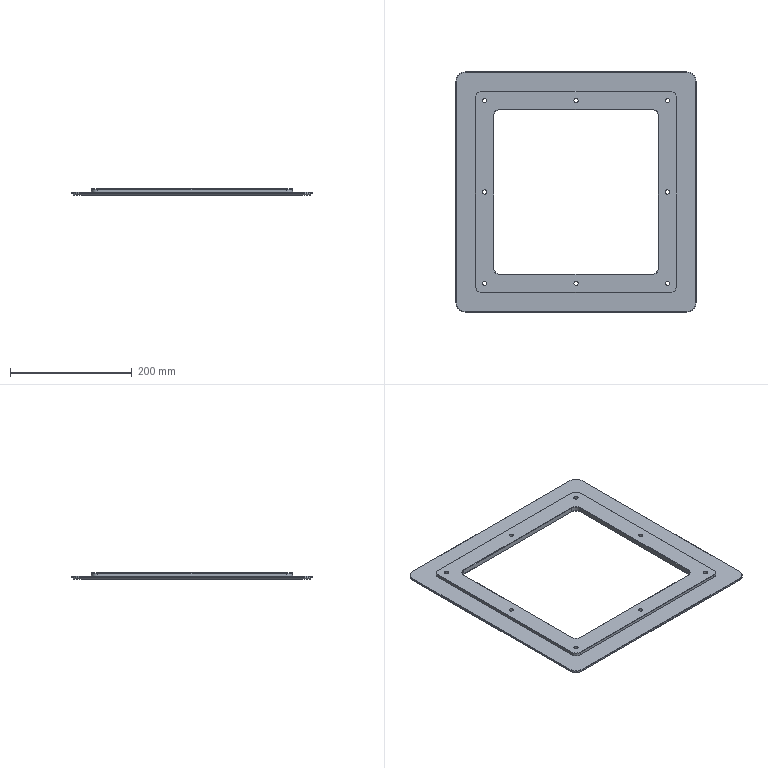NC program | Mastercam | posted with a generic post
Lines 951 to 2441 of 5147:
N9520 T14 M6
N9530 G0 G90 G17 G54 X-266.551 Y206.801 A0. S1600 M3
N9540 G43 H14 Z26.2 M8
N9550 Z11.2
N9560 G1 Z1.017 F1000.
N9570 X-208.008 Y207.805 F3200.
N9580 X208.008
N9590 Y194.817
N9600 X-208.008
N9610 Y181.829
N9620 X208.008
N9630 Y168.841
N9640 X-208.008
N9650 Y155.854
N9660 X208.008
N9670 Y142.866
N9680 X-208.008
N9690 Y129.878
N9700 X208.008
N9710 Y116.89
N9720 X-208.008
N9730 Y103.902
N9740 X-114.974
N9750 G3 X-121.856 Y90.915 I19.974 J-18.902
N9760 G1 X-208.008
N9770 Y77.927
N9780 X-121.575
N9790 G3 X-113.81 Y64.939 I26.575 J7.073
N9800 G1 X-208.008
N9810 Y51.951
N9820 X208.008
N9830 Y38.963
N9840 X-208.008
N9850 Y25.976
N9860 X208.008
N9870 Y12.988
N9880 X-208.008
N9890 Y0.
N9900 X208.008
N9910 Y-12.988
N9920 X-208.008
N9930 Y-25.976
N9940 X208.008
N9950 Y-38.963
N9960 X-208.008
N9970 Y-51.951
N9980 X208.008
N9990 Y-64.939
N100 X113.81
N110 G2 X121.575 Y-77.927 I-18.81 J-20.061
N120 G1 X208.008
N130 Y-90.915
N140 X121.856
N150 G2 X114.974 Y-103.902 I-26.856 J5.915
N160 G1 X208.008
N170 Y-116.89
N180 X-208.008
N190 Y-129.878
N200 X208.008
N210 Y-142.866
N220 X-208.008
N230 Y-155.854
N240 X208.008
N250 Y-168.841
N260 X-208.008
N270 Y-181.829
N280 X208.008
N290 Y-194.817
N300 X-208.008
N310 Y-207.805
N320 X208.008
N330 X81.49 Y-108.953
N340 G2 X75.026 Y-103.902 I13.51 J23.953
N350 G1 X-75.026
N360 G3 X-68.144 Y-90.915 I-19.974 J18.902
N370 G1 X68.144
N380 G2 X67.5 Y-85. I26.856 J5.915
N390 X68.425 Y-77.927 I27.5 J0.
N400 G1 X-68.425
N410 G3 X-76.19 Y-64.939 I-26.575 J-7.073
N420 G1 X76.19
N430 Y64.939
N440 X-76.19
N450 G3 X-68.425 Y77.927 I-18.81 J20.061
N460 G1 X68.425
N470 G2 X67.5 Y85. I26.575 J7.073
N480 X68.144 Y90.915 I27.5 J0.
N490 G1 X-68.144
N500 G3 X-75.026 Y103.902 I-26.856 J-5.915
N510 G1 X75.026
N520 G2 X95. Y112.5 I19.974 J-18.902
N530 X114.974 Y103.902 I0. J-27.5
N540 G1 X208.008
N550 Y90.915
N560 X121.856
N570 G2 X122.5 Y85. I-26.856 J-5.915
N580 X121.575 Y77.927 I-27.5 J0.
N590 G1 X208.008
N600 Y64.939
N610 X113.81
N620 G2 X108.624 Y61.112 I-18.81 J20.061
N630 G1 X-71.049 Y-71.486
N640 G3 X-95. Y-57.499 I-23.951 J-13.514
N650 X-122.501 Y-85. I0. J-27.501
N660 X-114.974 Y-103.902 I27.501 J0.
N670 G1 X-208.008
N680 Y-90.915
N690 X-121.856
N700 G2 X-122.5 Y-85. I26.856 J5.915
N710 X-121.575 Y-77.927 I27.5 J0.
N720 G1 X-208.008
N730 Y-64.939
N740 X-113.81
N750 G0 Z26.017
N760 X-266.551 Y206.801
N770 Z11.017
N780 G1 Z.833 F1000.
N790 X-208.008 Y207.805 F3200.
N800 X208.008
N810 Y194.817
N820 X-208.008
N830 Y181.829
N840 X208.008
N850 Y168.841
N860 X-208.008
N870 Y155.854
N880 X208.008
N890 Y142.866
N900 X-208.008
N910 Y129.878
N920 X208.008
N930 Y116.89
N940 X-208.008
N950 Y103.902
N960 X-114.974
N970 G3 X-121.856 Y90.915 I19.974 J-18.902
N980 G1 X-208.008
N990 Y77.927
N1000 X-121.575
N1010 G3 X-113.81 Y64.939 I26.575 J7.073
N1020 G1 X-208.008
N1030 Y51.951
N1040 X208.008
N1050 Y38.963
N1060 X-208.008
N1070 Y25.976
N1080 X208.008
N1090 Y12.988
N1100 X-208.008
N1110 Y0.
N1120 X208.008
N1130 Y-12.988
N1140 X-208.008
N1150 Y-25.976
N1160 X208.008
N1170 Y-38.963
N1180 X-208.008
N1190 Y-51.951
N1200 X208.008
N1210 Y-64.939
N1220 X113.81
N1230 G2 X121.575 Y-77.927 I-18.81 J-20.061
N1240 G1 X208.008
N1250 Y-90.915
N1260 X121.856
N1270 G2 X114.974 Y-103.902 I-26.856 J5.915
N1280 G1 X208.008
N1290 Y-116.89
N1300 X-208.008
N1310 Y-129.878
N1320 X208.008
N1330 Y-142.866
N1340 X-208.008
N1350 Y-155.854
N1360 X208.008
N1370 Y-168.841
N1380 X-208.008
N1390 Y-181.829
N1400 X208.008
N1410 Y-194.817
N1420 X-208.008
N1430 Y-207.805
N1440 X208.008
N1450 X81.49 Y-108.953
N1460 G2 X75.026 Y-103.902 I13.51 J23.953
N1470 G1 X-75.026
N1480 G3 X-68.144 Y-90.915 I-19.974 J18.902
N1490 G1 X68.144
N1500 G2 X67.5 Y-85. I26.856 J5.915
N1510 X68.425 Y-77.927 I27.5 J0.
N1520 G1 X-68.425
N1530 G3 X-76.19 Y-64.939 I-26.575 J-7.073
N1540 G1 X76.19
N1550 Y64.939
N1560 X-76.19
N1570 G3 X-68.425 Y77.927 I-18.81 J20.061
N1580 G1 X68.425
N1590 G2 X67.5 Y85. I26.575 J7.073
N1600 X68.144 Y90.915 I27.5 J0.
N1610 G1 X-68.144
N1620 G3 X-75.026 Y103.902 I-26.856 J-5.915
N1630 G1 X75.026
N1640 G2 X95. Y112.5 I19.974 J-18.902
N1650 X114.974 Y103.902 I0. J-27.5
N1660 G1 X208.008
N1670 Y90.915
N1680 X121.856
N1690 G2 X122.5 Y85. I-26.856 J-5.915
N1700 X121.575 Y77.927 I-27.5 J0.
N1710 G1 X208.008
N1720 Y64.939
N1730 X113.81
N1740 G2 X108.624 Y61.112 I-18.81 J20.061
N1750 G1 X-71.049 Y-71.486
N1760 G3 X-95. Y-57.499 I-23.951 J-13.514
N1770 X-122.501 Y-85. I0. J-27.501
N1780 X-114.974 Y-103.902 I27.501 J0.
N1790 G1 X-208.008
N1800 Y-90.915
N1810 X-121.856
N1820 G2 X-122.5 Y-85. I26.856 J5.915
N1830 X-121.575 Y-77.927 I27.5 J0.
N1840 G1 X-208.008
N1850 Y-64.939
N1860 X-113.81
N1870 G0 Z25.833
N1880 X-266.551 Y206.801
N1890 Z10.833
N1900 G1 Z.65 F1000.
N1910 X-208.008 Y207.805 F3200.
N1920 X208.008
N1930 Y194.817
N1940 X-208.008
N1950 Y181.829
N1960 X208.008
N1970 Y168.841
N1980 X-208.008
N1990 Y155.854
N2000 X208.008
N2010 Y142.866
N2020 X-208.008
N2030 Y129.878
N2040 X208.008
N2050 Y116.89
N2060 X-208.008
N2070 Y103.902
N2080 X-114.974
N2090 G3 X-121.856 Y90.915 I19.974 J-18.902
N2100 G1 X-208.008
N2110 Y77.927
N2120 X-121.575
N2130 G3 X-113.81 Y64.939 I26.575 J7.073
N2140 G1 X-208.008
N2150 Y51.951
N2160 X208.008
N2170 Y38.963
N2180 X-208.008
N2190 Y25.976
N2200 X208.008
N2210 Y12.988
N2220 X-208.008
N2230 Y0.
N2240 X208.008
N2250 Y-12.988
N2260 X-208.008
N2270 Y-25.976
N2280 X208.008
N2290 Y-38.963
N2300 X-208.008
N2310 Y-51.951
N2320 X208.008
N2330 Y-64.939
N2340 X113.81
N2350 G2 X121.575 Y-77.927 I-18.81 J-20.061
N2360 G1 X208.008
N2370 Y-90.915
N2380 X121.856
N2390 G2 X114.974 Y-103.902 I-26.856 J5.915
N2400 G1 X208.008
N2410 Y-116.89
N2420 X-208.008
N2430 Y-129.878
N2440 X208.008
N2450 Y-142.866
N2460 X-208.008
N2470 Y-155.854
N2480 X208.008
N2490 Y-168.841
N2500 X-208.008
N2510 Y-181.829
N2520 X208.008
N2530 Y-194.817
N2540 X-208.008
N2550 Y-207.805
N2560 X208.008
N2570 X81.49 Y-108.953
N2580 G2 X75.026 Y-103.902 I13.51 J23.953
N2590 G1 X-75.026
N2600 G3 X-68.144 Y-90.915 I-19.974 J18.902
N2610 G1 X68.144
N2620 G2 X67.5 Y-85. I26.856 J5.915
N2630 X68.425 Y-77.927 I27.5 J0.
N2640 G1 X-68.425
N2650 G3 X-76.19 Y-64.939 I-26.575 J-7.073
N2660 G1 X76.19
N2670 Y64.939
N2680 X-76.19
N2690 G3 X-68.425 Y77.927 I-18.81 J20.061
N2700 G1 X68.425
N2710 G2 X67.5 Y85. I26.575 J7.073
N2720 X68.144 Y90.915 I27.5 J0.
N2730 G1 X-68.144
N2740 G3 X-75.026 Y103.902 I-26.856 J-5.915
N2750 G1 X75.026
N2760 G2 X95. Y112.5 I19.974 J-18.902
N2770 X114.974 Y103.902 I0. J-27.5
N2780 G1 X208.008
N2790 Y90.915
N2800 X121.856
N2810 G2 X122.5 Y85. I-26.856 J-5.915
N2820 X121.575 Y77.927 I-27.5 J0.
N2830 G1 X208.008
N2840 Y64.939
N2850 X113.81
N2860 G2 X108.624 Y61.112 I-18.81 J20.061
N2870 G1 X-71.049 Y-71.486
N2880 G3 X-95. Y-57.499 I-23.951 J-13.514
N2890 X-122.501 Y-85. I0. J-27.501
N2900 X-114.974 Y-103.902 I27.501 J0.
N2910 G1 X-208.008
N2920 Y-90.915
N2930 X-121.856
N2940 G2 X-122.5 Y-85. I26.856 J5.915
N2950 X-121.575 Y-77.927 I27.5 J0.
N2960 G1 X-208.008
N2970 Y-64.939
N2980 X-113.81
N2990 G0 Z25.65
N3000 X-266.551 Y206.801
N3010 Z10.65
N3020 G1 Z.467 F1000.
N3030 X-208.008 Y207.805 F3200.
N3040 X208.008
N3050 Y194.817
N3060 X-208.008
N3070 Y181.829
N3080 X208.008
N3090 Y168.841
N3100 X-208.008
N3110 Y155.854
N3120 X208.008
N3130 Y142.866
N3140 X-208.008
N3150 Y129.878
N3160 X208.008
N3170 Y116.89
N3180 X-208.008
N3190 Y103.902
N3200 X-114.974
N3210 G3 X-121.856 Y90.915 I19.974 J-18.902
N3220 G1 X-208.008
N3230 Y77.927
N3240 X-121.575
N3250 G3 X-113.81 Y64.939 I26.575 J7.073
N3260 G1 X-208.008
N3270 Y51.951
N3280 X208.008
N3290 Y38.963
N3300 X-208.008
N3310 Y25.976
N3320 X208.008
N3330 Y12.988
N3340 X-208.008
N3350 Y0.
N3360 X208.008
N3370 Y-12.988
N3380 X-208.008
N3390 Y-25.976
N3400 X208.008
N3410 Y-38.963
N3420 X-208.008
N3430 Y-51.951
N3440 X208.008
N3450 Y-64.939
N3460 X113.81
N3470 G2 X121.575 Y-77.927 I-18.81 J-20.061
N3480 G1 X208.008
N3490 Y-90.915
N3500 X121.856
N3510 G2 X114.974 Y-103.902 I-26.856 J5.915
N3520 G1 X208.008
N3530 Y-116.89
N3540 X-208.008
N3550 Y-129.878
N3560 X208.008
N3570 Y-142.866
N3580 X-208.008
N3590 Y-155.854
N3600 X208.008
N3610 Y-168.841
N3620 X-208.008
N3630 Y-181.829
N3640 X208.008
N3650 Y-194.817
N3660 X-208.008
N3670 Y-207.805
N3680 X208.008
N3690 X81.49 Y-108.953
N3700 G2 X75.026 Y-103.902 I13.51 J23.953
N3710 G1 X-75.026
N3720 G3 X-68.144 Y-90.915 I-19.974 J18.902
N3730 G1 X68.144
N3740 G2 X67.5 Y-85. I26.856 J5.915
N3750 X68.425 Y-77.927 I27.5 J0.
N3760 G1 X-68.425
N3770 G3 X-76.19 Y-64.939 I-26.575 J-7.073
N3780 G1 X76.19
N3790 Y64.939
N3800 X-76.19
N3810 G3 X-68.425 Y77.927 I-18.81 J20.061
N3820 G1 X68.425
N3830 G2 X67.5 Y85. I26.575 J7.073
N3840 X68.144 Y90.915 I27.5 J0.
N3850 G1 X-68.144
N3860 G3 X-75.026 Y103.902 I-26.856 J-5.915
N3870 G1 X75.026
N3880 G2 X95. Y112.5 I19.974 J-18.902
N3890 X114.974 Y103.902 I0. J-27.5
N3900 G1 X208.008
N3910 Y90.915
N3920 X121.856
N3930 G2 X122.5 Y85. I-26.856 J-5.915
N3940 X121.575 Y77.927 I-27.5 J0.
N3950 G1 X208.008
N3960 Y64.939
N3970 X113.81
N3980 G2 X108.624 Y61.112 I-18.81 J20.061
N3990 G1 X-71.049 Y-71.486
N4000 G3 X-95. Y-57.499 I-23.951 J-13.514
N4010 X-122.501 Y-85. I0. J-27.501
N4020 X-114.974 Y-103.902 I27.501 J0.
N4030 G1 X-208.008
N4040 Y-90.915
N4050 X-121.856
N4060 G2 X-122.5 Y-85. I26.856 J5.915
N4070 X-121.575 Y-77.927 I27.5 J0.
N4080 G1 X-208.008
N4090 Y-64.939
N4100 X-113.81
N4110 G0 Z25.467
N4120 X-266.551 Y206.801
N4130 Z10.467
N4140 G1 Z.283 F1000.
N4150 X-208.008 Y207.805 F3200.
N4160 X208.008
N4170 Y194.817
N4180 X-208.008
N4190 Y181.829
N4200 X208.008
N4210 Y168.841
N4220 X-208.008
N4230 Y155.854
N4240 X208.008
N4250 Y142.866
N4260 X-208.008
N4270 Y129.878
N4280 X208.008
N4290 Y116.89
N4300 X-208.008
N4310 Y103.902
N4320 X-114.974
N4330 G3 X-121.856 Y90.915 I19.974 J-18.902
N4340 G1 X-208.008
N4350 Y77.927
N4360 X-121.575
N4370 G3 X-113.81 Y64.939 I26.575 J7.073
N4380 G1 X-208.008
N4390 Y51.951
N4400 X208.008
N4410 Y38.963
N4420 X-208.008
N4430 Y25.976
N4440 X208.008
N4450 Y12.988
N4460 X-208.008
N4470 Y0.
N4480 X208.008
N4490 Y-12.988
N4500 X-208.008
N4510 Y-25.976
N4520 X208.008
N4530 Y-38.963
N4540 X-208.008
N4550 Y-51.951
N4560 X208.008
N4570 Y-64.939
N4580 X113.81
N4590 G2 X121.575 Y-77.927 I-18.81 J-20.061
N4600 G1 X208.008
N4610 Y-90.915
N4620 X121.856
N4630 G2 X114.974 Y-103.902 I-26.856 J5.915
N4640 G1 X208.008
N4650 Y-116.89
N4660 X-208.008
N4670 Y-129.878
N4680 X208.008
N4690 Y-142.866
N4700 X-208.008
N4710 Y-155.854
N4720 X208.008
N4730 Y-168.841
N4740 X-208.008
N4750 Y-181.829
N4760 X208.008
N4770 Y-194.817
N4780 X-208.008
N4790 Y-207.805
N4800 X208.008
N4810 X81.49 Y-108.953
N4820 G2 X75.026 Y-103.902 I13.51 J23.953
N4830 G1 X-75.026
N4840 G3 X-68.144 Y-90.915 I-19.974 J18.902
N4850 G1 X68.144
N4860 G2 X67.5 Y-85. I26.856 J5.915
N4870 X68.425 Y-77.927 I27.5 J0.
N4880 G1 X-68.425
N4890 G3 X-76.19 Y-64.939 I-26.575 J-7.073
N4900 G1 X76.19
N4910 Y64.939
N4920 X-76.19
N4930 G3 X-68.425 Y77.927 I-18.81 J20.061
N4940 G1 X68.425
N4950 G2 X67.5 Y85. I26.575 J7.073
N4960 X68.144 Y90.915 I27.5 J0.
N4970 G1 X-68.144
N4980 G3 X-75.026 Y103.902 I-26.856 J-5.915
N4990 G1 X75.026
N5000 G2 X95. Y112.5 I19.974 J-18.902
N5010 X114.974 Y103.902 I0. J-27.5
N5020 G1 X208.008
N5030 Y90.915
N5040 X121.856
N5050 G2 X122.5 Y85. I-26.856 J-5.915
N5060 X121.575 Y77.927 I-27.5 J0.
N5070 G1 X208.008
N5080 Y64.939
N5090 X113.81
N5100 G2 X108.624 Y61.112 I-18.81 J20.061
N5110 G1 X-71.049 Y-71.486
N5120 G3 X-95. Y-57.499 I-23.951 J-13.514
N5130 X-122.501 Y-85. I0. J-27.501
N5140 X-114.974 Y-103.902 I27.501 J0.
N5150 G1 X-208.008
N5160 Y-90.915
N5170 X-121.856
N5180 G2 X-122.5 Y-85. I26.856 J5.915
N5190 X-121.575 Y-77.927 I27.5 J0.
N5200 G1 X-208.008
N5210 Y-64.939
N5220 X-113.81
N5230 G0 Z25.283
N5240 X-266.551 Y206.801
N5250 Z10.283
N5260 G1 Z.1 F1000.
N5270 X-208.008 Y207.805 F3200.
N5280 X208.008
N5290 Y194.817
N5300 X-208.008
N5310 Y181.829
N5320 X208.008
N5330 Y168.841
N5340 X-208.008
N5350 Y155.854
N5360 X208.008
N5370 Y142.866
N5380 X-208.008
N5390 Y129.878
N5400 X208.008
N5410 Y116.89
N5420 X-208.008
N5430 Y103.902
N5440 X-114.974
N5450 G3 X-121.856 Y90.915 I19.974 J-18.902
N5460 G1 X-208.008
N5470 Y77.927
N5480 X-121.575
N5490 G3 X-113.81 Y64.939 I26.575 J7.073
N5500 G1 X-208.008
N5510 Y51.951
N5520 X208.008
N5530 Y38.963
N5540 X-208.008
N5550 Y25.976
N5560 X208.008
N5570 Y12.988
N5580 X-208.008
N5590 Y0.
N5600 X208.008
N5610 Y-12.988
N5620 X-208.008
N5630 Y-25.976
N5640 X208.008
N5650 Y-38.963
N5660 X-208.008
N5670 Y-51.951
N5680 X208.008
N5690 Y-64.939
N5700 X113.81
N5710 G2 X121.575 Y-77.927 I-18.81 J-20.061
N5720 G1 X208.008
N5730 Y-90.915
N5740 X121.856
N5750 G2 X114.974 Y-103.902 I-26.856 J5.915
N5760 G1 X208.008
N5770 Y-116.89
N5780 X-208.008
N5790 Y-129.878
N5800 X208.008
N5810 Y-142.866
N5820 X-208.008
N5830 Y-155.854
N5840 X208.008
N5850 Y-168.841
N5860 X-208.008
N5870 Y-181.829
N5880 X208.008
N5890 Y-194.817
N5900 X-208.008
N5910 Y-207.805
N5920 X208.008
N5930 X81.49 Y-108.953
N5940 G2 X75.026 Y-103.902 I13.51 J23.953
N5950 G1 X-75.026
N5960 G3 X-68.144 Y-90.915 I-19.974 J18.902
N5970 G1 X68.144
N5980 G2 X67.5 Y-85. I26.856 J5.915
N5990 X68.425 Y-77.927 I27.5 J0.
N6000 G1 X-68.425
N6010 G3 X-76.19 Y-64.939 I-26.575 J-7.073
N6020 G1 X76.19
N6030 Y64.939
N6040 X-76.19
N6050 G3 X-68.425 Y77.927 I-18.81 J20.061
N6060 G1 X68.425
N6070 G2 X67.5 Y85. I26.575 J7.073
N6080 X68.144 Y90.915 I27.5 J0.
N6090 G1 X-68.144
N6100 G3 X-75.026 Y103.902 I-26.856 J-5.915
N6110 G1 X75.026
N6120 G2 X95. Y112.5 I19.974 J-18.902
N6130 X114.974 Y103.902 I0. J-27.5
N6140 G1 X208.008
N6150 Y90.915
N6160 X121.856
N6170 G2 X122.5 Y85. I-26.856 J-5.915
N6180 X121.575 Y77.927 I-27.5 J0.
N6190 G1 X208.008
N6200 Y64.939
N6210 X113.81
N6220 G2 X108.624 Y61.112 I-18.81 J20.061
N6230 G1 X-71.049 Y-71.486
N6240 G3 X-95. Y-57.499 I-23.951 J-13.514
N6250 X-122.501 Y-85. I0. J-27.501
N6260 X-114.974 Y-103.902 I27.501 J0.
N6270 G1 X-208.008
N6280 Y-90.915
N6290 X-121.856
N6300 G2 X-122.5 Y-85. I26.856 J5.915
N6310 X-121.575 Y-77.927 I27.5 J0.
N6320 G1 X-208.008
N6330 Y-64.939
N6340 X-113.81
N6350 G0 Z26.2
N6360 X-66.5 Y87. Z50.
N6370 Z2.2
N6380 G1 Z1.2 F600.
N6390 X-68.5 F3000.
N6400 G3 X-70.5 Y85. I0. J-2.
N6410 G2 X-95. Y60.5 Z1.125 I-24.5 J0.
N6420 X-119.5 Y85. Z1.05 I0. J24.5
N6430 X-95. Y109.5 Z.975 I24.5 J0.
N6440 X-70.5 Y85. Z.9 I0. J-24.5
N6450 X-95. Y60.5 Z.825 I-24.5 J0.
N6460 X-119.5 Y85. Z.75 I0. J24.5
N6470 X-95. Y109.5 Z.675 I24.5 J0.
N6480 X-70.5 Y85. Z.6 I0. J-24.5
N6490 X-95. Y60.5 Z.525 I-24.5 J0.
N6500 X-119.5 Y85. Z.45 I0. J24.5
N6510 X-95. Y109.5 Z.375 I24.5 J0.
N6520 X-70.5 Y85. Z.3 I0. J-24.5
N6530 X-95. Y60.5 Z.225 I-24.5 J0.
N6540 X-119.5 Y85. Z.15 I0. J24.5
N6550 X-107.25 Y106.218 Z.1 I24.5 J0.
N6560 X-95. Y109.5 I12.25 J-21.218
N6570 X-70.5 Y85. I0. J-24.5
N6580 X-95. Y60.5 I-24.5 J0.
N6590 X-119.5 Y85. I0. J24.5
N6600 X-107.25 Y106.218 I24.5 J0.
N6610 G3 X-106.25 Y107.95 I-1. J1.732
N6620 X-106.518 Y108.95 I-2. J0.
N6630 G1 X-107.518 Y110.682
N6640 G0 Z50.
N6650 X-66.5 Y-83.
N6660 Z2.2
N6670 G1 Z1.2 F600.
N6680 X-68.5 F3000.
N6690 G3 X-70.5 Y-85. I0. J-2.
N6700 G2 X-95. Y-109.5 Z1.125 I-24.5 J0.
N6710 X-119.5 Y-85. Z1.05 I0. J24.5
N6720 X-95. Y-60.5 Z.975 I24.5 J0.
N6730 X-70.5 Y-85. Z.9 I0. J-24.5
N6740 X-95. Y-109.5 Z.825 I-24.5 J0.
N6750 X-119.5 Y-85. Z.75 I0. J24.5
N6760 X-95. Y-60.5 Z.675 I24.5 J0.
N6770 X-70.5 Y-85. Z.6 I0. J-24.5
N6780 X-95. Y-109.5 Z.525 I-24.5 J0.
N6790 X-119.5 Y-85. Z.45 I0. J24.5
N6800 X-95. Y-60.5 Z.375 I24.5 J0.
N6810 X-70.5 Y-85. Z.3 I0. J-24.5
N6820 X-95. Y-109.5 Z.225 I-24.5 J0.
N6830 X-119.5 Y-85. Z.15 I0. J24.5
N6840 X-107.25 Y-63.782 Z.1 I24.5 J0.
N6850 X-95. Y-60.5 I12.25 J-21.218
N6860 X-70.5 Y-85. I0. J-24.5
N6870 X-95. Y-109.5 I-24.5 J0.
N6880 X-119.5 Y-85. I0. J24.5
N6890 X-107.25 Y-63.782 I24.5 J0.
N6900 G3 X-106.25 Y-62.05 I-1. J1.732
N6910 X-106.518 Y-61.05 I-2. J0.
N6920 G1 X-107.518 Y-59.318
N6930 G0 Z50.
N6940 X123.5 Y-83.
N6950 Z2.2
N6960 G1 Z1.2 F600.
N6970 X121.5 F3000.
N6980 G3 X119.5 Y-85. I0. J-2.
N6990 G2 X95. Y-109.5 Z1.125 I-24.5 J0.
N7000 X70.5 Y-85. Z1.05 I0. J24.5
N7010 X95. Y-60.5 Z.975 I24.5 J0.
N7020 X119.5 Y-85. Z.9 I0. J-24.5
N7030 X95. Y-109.5 Z.825 I-24.5 J0.
N7040 X70.5 Y-85. Z.75 I0. J24.5
N7050 X95. Y-60.5 Z.675 I24.5 J0.
N7060 X119.5 Y-85. Z.6 I0. J-24.5
N7070 X95. Y-109.5 Z.525 I-24.5 J0.
N7080 X70.5 Y-85. Z.45 I0. J24.5
N7090 X95. Y-60.5 Z.375 I24.5 J0.
N7100 X119.5 Y-85. Z.3 I0. J-24.5
N7110 X95. Y-109.5 Z.225 I-24.5 J0.
N7120 X70.5 Y-85. Z.15 I0. J24.5
N7130 X82.75 Y-63.782 Z.1 I24.5 J0.
N7140 X95. Y-60.5 I12.25 J-21.218
N7150 X119.5 Y-85. I0. J-24.5
N7160 X95. Y-109.5 I-24.5 J0.
N7170 X70.5 Y-85. I0. J24.5
N7180 X82.75 Y-63.782 I24.5 J0.
N7190 G3 X83.75 Y-62.05 I-1. J1.732
N7200 X83.482 Y-61.05 I-2. J0.
N7210 G1 X82.482 Y-59.318
N7220 G0 Z50.
N7230 X123.5 Y87.
N7240 Z2.2
N7250 G1 Z1.2 F600.
N7260 X121.5 F3000.
N7270 G3 X119.5 Y85. I0. J-2.
N7280 G2 X95. Y60.5 Z1.125 I-24.5 J0.
N7290 X70.5 Y85. Z1.05 I0. J24.5
N7300 X95. Y109.5 Z.975 I24.5 J0.
N7310 X119.5 Y85. Z.9 I0. J-24.5
N7320 X95. Y60.5 Z.825 I-24.5 J0.
N7330 X70.5 Y85. Z.75 I0. J24.5
N7340 X95. Y109.5 Z.675 I24.5 J0.
N7350 X119.5 Y85. Z.6 I0. J-24.5
N7360 X95. Y60.5 Z.525 I-24.5 J0.
N7370 X70.5 Y85. Z.45 I0. J24.5
N7380 X95. Y109.5 Z.375 I24.5 J0.
N7390 X119.5 Y85. Z.3 I0. J-24.5
N7400 X95. Y60.5 Z.225 I-24.5 J0.
N7410 X70.5 Y85. Z.15 I0. J24.5
N7420 X82.75 Y106.218 Z.1 I24.5 J0.
N7430 X95. Y109.5 I12.25 J-21.218
N7440 X119.5 Y85. I0. J-24.5
N7450 X95. Y60.5 I-24.5 J0.
N7460 X70.5 Y85. I0. J24.5
N7470 X82.75 Y106.218 I24.5 J0.
N7480 G3 X83.75 Y107.95 I-1. J1.732
N7490 X83.482 Y108.95 I-2. J0.
N7500 G1 X82.482 Y110.682
N7510 G0 Z50.
N7520 X-124.8 Y124.8
N7530 Z1.
N7540 G1 Z0. F600.
N7550 Y-124.8 Z-.075 F3000.
N7560 X124.8 Z-.15
N7570 Y124.8 Z-.225
N7580 X-124.8 Z-.3
N7590 Y-124.8 Z-.375
N7600 X124.8 Z-.45
N7610 Y124.8 Z-.525
N7620 X-124.8 Z-.6
N7630 Y-124.8 Z-.675
N7640 X124.8 Z-.75
N7650 Y124.8 Z-.825
N7660 X-124.8 Z-.9
N7670 Y-124.8 Z-.975
N7680 X124.8 Z-1.05
N7690 Y124.8 Z-1.125
N7700 X-124.8 Z-1.2
N7710 Y-124.8 Z-1.275
N7720 X124.8 Z-1.35
N7730 Y124.8 Z-1.425
N7740 X-124.8 Z-1.5
N7750 Y-124.8 Z-1.575
N7760 X124.8 Z-1.65
N7770 Y124.8 Z-1.725
N7780 X-124.8 Z-1.8
N7790 Y-124.8 Z-1.875
N7800 X124.8 Z-1.95
N7810 Y124.8 Z-2.025
N7820 X-124.8 Z-2.1
N7830 Y-124.8 Z-2.175
N7840 X124.8 Z-2.25
N7850 Y124.8 Z-2.325
N7860 X-124.8 Z-2.4
N7870 Y-124.8 Z-2.475
N7880 X124.8 Z-2.55
N7890 Y124.8 Z-2.625
N7900 X-124.8 Z-2.7
N7910 Y-124.8 Z-2.775
N7920 X124.8 Z-2.85
N7930 Y124.8 Z-2.925
N7940 X-124.8 Z-3.
N7950 Y-124.8
N7960 X124.8
N7970 Y124.8
N7980 X-124.8
N7990 G0 Z50.
N8000 S2000 M3
N8010 X-182. Y207.2
N8020 Z1.
N8030 G1 Z0. F600.
N8040 X182. Z-.068 F4000.
N8050 G2 X207.2 Y182. Z-.075 I0. J-25.2
N8060 G1 Y-182. Z-.143
N8070 G2 X182. Y-207.2 Z-.15 I-25.2 J0.
N8080 G1 X-182. Z-.218
N8090 G2 X-207.2 Y-182. Z-.225 I0. J25.2
N8100 G1 Y182. Z-.293
N8110 G2 X-182. Y207.2 Z-.3 I25.2 J0.
N8120 G1 X182. Z-.368
N8130 G2 X207.2 Y182. Z-.375 I0. J-25.2
N8140 G1 Y-182. Z-.443
N8150 G2 X182. Y-207.2 Z-.45 I-25.2 J0.
N8160 G1 X-182. Z-.518
N8170 G2 X-207.2 Y-182. Z-.525 I0. J25.2
N8180 G1 Y182. Z-.593
N8190 G2 X-182. Y207.2 Z-.6 I25.2 J0.
N8200 G1 X182. Z-.668
N8210 G2 X207.2 Y182. Z-.675 I0. J-25.2
N8220 G1 Y-182. Z-.743
N8230 G2 X182. Y-207.2 Z-.75 I-25.2 J0.
N8240 G1 X-182. Z-.818
N8250 G2 X-207.2 Y-182. Z-.825 I0. J25.2
N8260 G1 Y182. Z-.893
N8270 G2 X-182. Y207.2 Z-.9 I25.2 J0.
N8280 G1 X182. Z-.968
N8290 G2 X207.2 Y182. Z-.975 I0. J-25.2
N8300 G1 Y-182. Z-1.043
N8310 G2 X182. Y-207.2 Z-1.05 I-25.2 J0.
N8320 G1 X-182. Z-1.118
N8330 G2 X-207.2 Y-182. Z-1.125 I0. J25.2
N8340 G1 Y182. Z-1.193
N8350 G2 X-182. Y207.2 Z-1.2 I25.2 J0.
N8360 G1 X182. Z-1.268
N8370 G2 X207.2 Y182. Z-1.275 I0. J-25.2
N8380 G1 Y-182. Z-1.343
N8390 G2 X182. Y-207.2 Z-1.35 I-25.2 J0.
N8400 G1 X-182. Z-1.418
N8410 G2 X-207.2 Y-182. Z-1.425 I0. J25.2
N8420 G1 Y182. Z-1.493
N8430 G2 X-182. Y207.2 Z-1.5 I25.2 J0.
N8440 G1 X182. Z-1.568
N8450 G2 X207.2 Y182. Z-1.575 I0. J-25.2
N8460 G1 Y-182. Z-1.643
N8470 G2 X182. Y-207.2 Z-1.65 I-25.2 J0.
N8480 G1 X-182. Z-1.718
N8490 G2 X-207.2 Y-182. Z-1.725 I0. J25.2
N8500 G1 Y182. Z-1.793
N8510 G2 X-182. Y207.2 Z-1.8 I25.2 J0.
N8520 G1 X182. Z-1.868
N8530 G2 X207.2 Y182. Z-1.875 I0. J-25.2
N8540 G1 Y-182. Z-1.943
N8550 G2 X182. Y-207.2 Z-1.95 I-25.2 J0.
N8560 G1 X-182. Z-2.018
N8570 G2 X-207.2 Y-182. Z-2.025 I0. J25.2
N8580 G1 Y182. Z-2.093
N8590 G2 X-182. Y207.2 Z-2.1 I25.2 J0.
N8600 G1 X182. Z-2.168
N8610 G2 X207.2 Y182. Z-2.175 I0. J-25.2
N8620 G1 Y-182. Z-2.243
N8630 G2 X182. Y-207.2 Z-2.25 I-25.2 J0.
N8640 G1 X-182. Z-2.318
N8650 G2 X-207.2 Y-182. Z-2.325 I0. J25.2
N8660 G1 Y182. Z-2.393
N8670 G2 X-182. Y207.2 Z-2.4 I25.2 J0.
N8680 G1 X182. Z-2.468
N8690 G2 X207.2 Y182. Z-2.475 I0. J-25.2
N8700 G1 Y-182. Z-2.543
N8710 G2 X182. Y-207.2 Z-2.55 I-25.2 J0.
N8720 G1 X-182. Z-2.618
N8730 G2 X-207.2 Y-182. Z-2.625 I0. J25.2
N8740 G1 Y182. Z-2.693
N8750 G2 X-182. Y207.2 Z-2.7 I25.2 J0.
N8760 G1 X182. Z-2.768
N8770 G2 X207.2 Y182. Z-2.775 I0. J-25.2
N8780 G1 Y-182. Z-2.843
N8790 G2 X182. Y-207.2 Z-2.85 I-25.2 J0.
N8800 G1 X-182. Z-2.918
N8810 G2 X-207.2 Y-182. Z-2.925 I0. J25.2
N8820 G1 Y182. Z-2.993
N8830 G2 X-182. Y207.2 Z-3. I25.2 J0.
N8840 G1 X182. Z-3.068
N8850 G2 X207.2 Y182. Z-3.075 I0. J-25.2
N8860 G1 Y-182. Z-3.143
N8870 G2 X182. Y-207.2 Z-3.15 I-25.2 J0.
N8880 G1 X-182. Z-3.218
N8890 G2 X-207.2 Y-182. Z-3.225 I0. J25.2
N8900 G1 Y182. Z-3.293
N8910 G2 X-182. Y207.2 Z-3.3 I25.2 J0.
N8920 G1 X182. Z-3.368
N8930 G2 X207.2 Y182. Z-3.375 I0. J-25.2
N8940 G1 Y-182. Z-3.443
N8950 G2 X182. Y-207.2 Z-3.45 I-25.2 J0.
N8960 G1 X-182. Z-3.518
N8970 G2 X-207.2 Y-182. Z-3.525 I0. J25.2
N8980 G1 Y182. Z-3.593
N8990 G2 X-182. Y207.2 Z-3.6 I25.2 J0.
N9000 G1 X182. Z-3.668
N9010 G2 X207.2 Y182. Z-3.675 I0. J-25.2
N9020 G1 Y-182. Z-3.743
N9030 G2 X182. Y-207.2 Z-3.75 I-25.2 J0.
N9040 G1 X-182. Z-3.818
N9050 G2 X-207.2 Y-182. Z-3.825 I0. J25.2
N9060 G1 Y182. Z-3.893
N9070 G2 X-182. Y207.2 Z-3.9 I25.2 J0.
N9080 G1 X182. Z-3.968
N9090 G2 X207.2 Y182. Z-3.975 I0. J-25.2
N9100 G1 Y-182. Z-4.043
N9110 G2 X182. Y-207.2 Z-4.05 I-25.2 J0.
N9120 G1 X-182. Z-4.118
N9130 G2 X-207.2 Y-182. Z-4.125 I0. J25.2
N9140 G1 Y182. Z-4.193
N9150 G2 X-182. Y207.2 Z-4.2 I25.2 J0.
N9160 G1 X182. Z-4.268
N9170 G2 X207.2 Y182. Z-4.275 I0. J-25.2
N9180 G1 Y-182. Z-4.343
N9190 G2 X182. Y-207.2 Z-4.35 I-25.2 J0.
N9200 G1 X-182. Z-4.418
N9210 G2 X-207.2 Y-182. Z-4.425 I0. J25.2
N9220 G1 Y182. Z-4.493
N9230 G2 X-182. Y207.2 Z-4.5 I25.2 J0.
N9240 G1 X182. Z-4.568
N9250 G2 X207.2 Y182. Z-4.575 I0. J-25.2
N9260 G1 Y-182. Z-4.643
N9270 G2 X182. Y-207.2 Z-4.65 I-25.2 J0.
N9280 G1 X-182. Z-4.718
N9290 G2 X-207.2 Y-182. Z-4.725 I0. J25.2
N9300 G1 Y182. Z-4.793
N9310 G2 X-182. Y207.2 Z-4.8 I25.2 J0.
N9320 G1 X182. Z-4.868
N9330 G2 X207.2 Y182. Z-4.875 I0. J-25.2
N9340 G1 Y-182. Z-4.943
N9350 G2 X182. Y-207.2 Z-4.95 I-25.2 J0.
N9360 G1 X-182. Z-5.018
N9370 G2 X-207.2 Y-182. Z-5.025 I0. J25.2
N9380 G1 Y182. Z-5.093
N9390 G2 X-182. Y207.2 Z-5.1 I25.2 J0.
N9400 G1 X182. Z-5.168
N9410 G2 X207.2 Y182. Z-5.175 I0. J-25.2
N9420 G1 Y-182. Z-5.243
N9430 G2 X182. Y-207.2 Z-5.25 I-25.2 J0.
N9440 G1 X-182. Z-5.318
N9450 G2 X-207.2 Y-182. Z-5.325 I0. J25.2
N9460 G1 Y182. Z-5.393
N9470 G2 X-182. Y207.2 Z-5.4 I25.2 J0.
N9480 G1 X182. Z-5.468
N9490 G2 X207.2 Y182. Z-5.475 I0. J-25.2
N9500 G1 Y-182. Z-5.543
N9510 G2 X182. Y-207.2 Z-5.55 I-25.2 J0.
N9520 G1 X-182. Z-5.618
N9530 G2 X-207.2 Y-182. Z-5.625 I0. J25.2
N9540 G1 Y182. Z-5.693
N9550 G2 X-182. Y207.2 Z-5.7 I25.2 J0.
N9560 G1 X182. Z-5.768
N9570 G2 X207.2 Y182. Z-5.775 I0. J-25.2
N9580 G1 Y-182. Z-5.843
N9590 G2 X182. Y-207.2 Z-5.85 I-25.2 J0.
N9600 G1 X-182. Z-5.918
N9610 G2 X-207.2 Y-182. Z-5.925 I0. J25.2
N9620 G1 Y182. Z-5.993
N9630 G2 X-182. Y207.2 Z-6. I25.2 J0.
N9640 G1 X182. Z-6.068
N9650 G2 X207.2 Y182. Z-6.075 I0. J-25.2
N9660 G1 Y-182. Z-6.143
N9670 G2 X182. Y-207.2 Z-6.15 I-25.2 J0.
N9680 G1 X-182. Z-6.218
N9690 G2 X-207.2 Y-182. Z-6.225 I0. J25.2
N9700 G1 Y182. Z-6.293
N9710 G2 X-182. Y207.2 Z-6.3 I25.2 J0.
N9720 G1 X182. Z-6.368
N9730 G2 X207.2 Y182. Z-6.375 I0. J-25.2
N9740 G1 Y-182. Z-6.443
N9750 G2 X182. Y-207.2 Z-6.45 I-25.2 J0.
N9760 G1 X-182. Z-6.518
N9770 G2 X-207.2 Y-182. Z-6.525 I0. J25.2
N9780 G1 Y182. Z-6.593
N9790 G2 X-182. Y207.2 Z-6.6 I25.2 J0.
N9800 G1 X182. Z-6.668
N9810 G2 X207.2 Y182. Z-6.675 I0. J-25.2
N9820 G1 Y-182. Z-6.743
N9830 G2 X182. Y-207.2 Z-6.75 I-25.2 J0.
N9840 G1 X-182. Z-6.818
N9850 G2 X-207.2 Y-182. Z-6.825 I0. J25.2
N9860 G1 Y182. Z-6.893
N9870 G2 X-182. Y207.2 Z-6.9 I25.2 J0.
N9880 G1 X182. Z-6.968
N9890 G2 X207.2 Y182. Z-6.975 I0. J-25.2
N9900 G1 Y-182. Z-7.043
N9910 G2 X182. Y-207.2 Z-7.05 I-25.2 J0.
N9920 G1 X-182. Z-7.118
N9930 G2 X-207.2 Y-182. Z-7.125 I0. J25.2
N9940 G1 Y182. Z-7.193
N9950 G2 X-182. Y207.2 Z-7.2 I25.2 J0.
N9960 G1 X182. Z-7.268
N9970 G2 X207.2 Y182. Z-7.275 I0. J-25.2
N9980 G1 Y-182. Z-7.343
N9990 G2 X182. Y-207.2 Z-7.35 I-25.2 J0.
N100 G1 X-182. Z-7.418
N110 G2 X-207.2 Y-182. Z-7.425 I0. J25.2
N120 G1 Y182. Z-7.493
N130 G2 X-182. Y207.2 Z-7.5 I25.2 J0.
N140 G1 X182. Z-7.568
N150 G2 X207.2 Y182. Z-7.575 I0. J-25.2
N160 G1 Y-182. Z-7.643
N170 G2 X182. Y-207.2 Z-7.65 I-25.2 J0.
N180 G1 X-182. Z-7.718
N190 G2 X-207.2 Y-182. Z-7.725 I0. J25.2
N200 G1 Y182. Z-7.793
N210 G2 X-182. Y207.2 Z-7.8 I25.2 J0.
N220 G1 X182. Z-7.868
N230 G2 X207.2 Y182. Z-7.875 I0. J-25.2
N240 G1 Y-182. Z-7.943
N250 G2 X182. Y-207.2 Z-7.95 I-25.2 J0.
N260 G1 X-182. Z-8.018
N270 G2 X-207.2 Y-182. Z-8.025 I0. J25.2
N280 G1 Y182. Z-8.093
N290 G2 X-182. Y207.2 Z-8.1 I25.2 J0.
N300 G1 X182. Z-8.168
N310 G2 X207.2 Y182. Z-8.175 I0. J-25.2
N320 G1 Y-182. Z-8.243
N330 G2 X182. Y-207.2 Z-8.25 I-25.2 J0.
N340 G1 X-182. Z-8.318
N350 G2 X-207.2 Y-182. Z-8.325 I0. J25.2
N360 G1 Y182. Z-8.393
N370 G2 X-182. Y207.2 Z-8.4 I25.2 J0.
N380 G1 X182. Z-8.468
N390 G2 X207.2 Y182. Z-8.475 I0. J-25.2
N400 G1 Y-182. Z-8.543
N410 G2 X182. Y-207.2 Z-8.55 I-25.2 J0.
N420 G1 X-182. Z-8.618
N430 G2 X-207.2 Y-182. Z-8.625 I0. J25.2
N440 G1 Y182. Z-8.693
N450 G2 X-182. Y207.2 Z-8.7 I25.2 J0.
N460 G1 X182. Z-8.768
N470 G2 X207.2 Y182. Z-8.775 I0. J-25.2
N480 G1 Y-182. Z-8.843
N490 G2 X182. Y-207.2 Z-8.85 I-25.2 J0.
N500 G1 X-182. Z-8.918
N510 G2 X-207.2 Y-182. Z-8.925 I0. J25.2
N520 G1 Y182. Z-8.993
N530 G2 X-182. Y207.2 Z-9. I25.2 J0.
N540 G1 X182. Z-9.068
N550 G2 X207.2 Y182. Z-9.075 I0. J-25.2
N560 G1 Y-182. Z-9.143
N570 G2 X182. Y-207.2 Z-9.15 I-25.2 J0.
N580 G1 X-182. Z-9.218
N590 G2 X-207.2 Y-182. Z-9.225 I0. J25.2
N600 G1 Y182. Z-9.293
N610 G2 X-182. Y207.2 Z-9.3 I25.2 J0.
N620 G1 X182. Z-9.368
N630 G2 X207.2 Y182. Z-9.375 I0. J-25.2
N640 G1 Y-182. Z-9.443
N650 G2 X182. Y-207.2 Z-9.45 I-25.2 J0.
N660 G1 X-182. Z-9.518
N670 G2 X-207.2 Y-182. Z-9.525 I0. J25.2
N680 G1 Y182. Z-9.593
N690 G2 X-182. Y207.2 Z-9.6 I25.2 J0.
N700 G1 X182. Z-9.668
N710 G2 X207.2 Y182. Z-9.675 I0. J-25.2
N720 G1 Y-182. Z-9.743
N730 G2 X182. Y-207.2 Z-9.75 I-25.2 J0.
N740 G1 X-182. Z-9.818
N750 G2 X-207.2 Y-182. Z-9.825 I0. J25.2
N760 G1 Y182. Z-9.893
N770 G2 X-182. Y207.2 Z-9.9 I25.2 J0.
N780 G1 X182. Z-9.968
N790 G2 X207.2 Y182. Z-9.975 I0. J-25.2
N800 G1 Y-182. Z-10.043
N810 G2 X182. Y-207.2 Z-10.05 I-25.2 J0.
N820 G1 X-182. Z-10.118
N830 G2 X-207.2 Y-182. Z-10.125 I0. J25.2
N840 G1 Y182. Z-10.193
N850 G2 X-182. Y207.2 Z-10.2 I25.2 J0.
N860 G1 X182. Z-10.268
N870 G2 X207.2 Y182. Z-10.275 I0. J-25.2
N880 G1 Y-182. Z-10.343
N890 G2 X182. Y-207.2 Z-10.35 I-25.2 J0.
N900 G1 X-182. Z-10.418
N910 G2 X-207.2 Y-182. Z-10.425 I0. J25.2
N920 G1 Y182. Z-10.493
N930 G2 X-182. Y207.2 Z-10.5 I25.2 J0.
N940 G1 X182. Z-10.568
N950 G2 X207.2 Y182. Z-10.575 I0. J-25.2
N960 G1 Y-182. Z-10.643
N970 G2 X182. Y-207.2 Z-10.65 I-25.2 J0.
N980 G1 X-182. Z-10.718
N990 G2 X-207.2 Y-182. Z-10.725 I0. J25.2
N1000 G1 Y182. Z-10.793
N1010 G2 X-182. Y207.2 Z-10.8 I25.2 J0.
N1020 G1 X182. Z-10.868
N1030 G2 X207.2 Y182. Z-10.875 I0. J-25.2
N1040 G1 Y-182. Z-10.943
N1050 G2 X182. Y-207.2 Z-10.95 I-25.2 J0.
N1060 G1 X-182. Z-11.018
N1070 G2 X-207.2 Y-182. Z-11.025 I0. J25.2
N1080 G1 Y182. Z-11.093
N1090 G2 X-182. Y207.2 Z-11.1 I25.2 J0.
N1100 G1 X182. Z-11.168
N1110 G2 X207.2 Y182. Z-11.175 I0. J-25.2
N1120 G1 Y-182. Z-11.243
N1130 G2 X182. Y-207.2 Z-11.25 I-25.2 J0.
N1140 G1 X-182. Z-11.318
N1150 G2 X-207.2 Y-182. Z-11.325 I0. J25.2
N1160 G1 Y182. Z-11.393
N1170 G2 X-182. Y207.2 Z-11.4 I25.2 J0.
N1180 G1 X182.
N1190 G2 X207.2 Y182. I0. J-25.2
N1200 G1 Y-182.
N1210 G2 X182. Y-207.2 I-25.2 J0.
N1220 G1 X-182.
N1230 G2 X-207.2 Y-182. I0. J25.2
N1240 G1 Y182.
N1250 G2 X-182. Y207.2 I25.2 J0.
N1260 G0 Z50.
N1270 M5
N1280 G91 G28 Z0. M9
N1290 A0.
N1300 M01
N1310 T12 M6
N1320 G0 G90 G17 G54 X-266.551 Y206.801 A0. S2000 M3
N1330 G43 H12 Z26.2 M8
N1340 Z11.2
N1350 G1 Z0. F600.
N1360 X-212.008 Y211.805 F800.
N1370 X212.008
N1380 Y204.103
N1390 X-212.008
N1400 Y196.401
N1410 X212.008
N1420 Y188.699
N1430 X-212.008
N1440 Y180.997
N1450 X212.008
N1460 Y173.295
N1470 X-212.008
N1480 Y165.593
N1490 X212.008
N1500 Y157.891
N1510 X-212.008
N1520 Y150.189
N1530 X212.008
N1540 Y142.487
N1550 X-212.008
N1560 Y134.785
N1570 X212.008
N1580 Y127.083
N1590 X-212.008
N1600 Y119.381
N1610 X212.008
N1620 Y111.679
N1630 X-212.008
N1640 Y103.977
N1650 X-108.861
N1660 G3 X-115.619 Y96.275 I13.861 J-18.977
N1670 G1 X-212.008
N1680 Y88.573
N1690 X-118.227
N1700 G3 X-118.5 Y85. I23.227 J-3.573
N1710 X-118.134 Y80.871 I23.5 J0.
N1720 G1 X-212.008
N1730 Y73.169
N1740 X-115.305
N1750 G3 X-108.066 Y65.467 I20.305 J11.831
N1760 G1 X-212.008
N1770 Y57.765
N1780 X212.008
N1790 Y50.063
N1800 X-212.008
N1810 Y42.361
N1820 X212.008
N1830 Y34.659
N1840 X-212.008
N1850 Y26.957
N1860 X212.008
N1870 Y19.255
N1880 X-212.008
N1890 Y11.553
N1900 X212.008
N1910 Y3.851
N1920 X-212.008
N1930 Y-3.851
N1940 X212.008
N1950 Y-11.553
N1960 X-212.008
N1970 Y-19.255
N1980 X212.008
N1990 Y-26.957
N2000 X-212.008
N2010 Y-34.659
N2020 X212.008
N2030 Y-42.361
N2040 X-212.008
N2050 Y-50.063
N2060 X212.008
N2070 Y-57.765
N2080 X-212.008
N2090 Y-65.467
N2100 X-108.066
N2110 G3 X-115.305 Y-73.169 I13.066 J-19.533
N2120 G1 X-212.008
N2130 Y-80.871
N2140 X-118.134
N2150 G3 X-118.5 Y-85. I23.134 J-4.129
N2160 X-118.227 Y-88.573 I23.5 J0.
N2170 G1 X-212.008
N2180 Y-96.275
N2190 X-115.619
N2200 G3 X-108.861 Y-103.977 I20.619 J11.275
N2210 G1 X-212.008
N2220 Y-111.679
N2230 X212.008
N2240 Y-119.381
N2250 X-212.008
N2260 Y-127.083
N2270 X212.008
N2280 Y-134.785
N2290 X-212.008
N2300 Y-142.487
N2310 X212.008
N2320 Y-150.189
N2330 X-212.008
N2340 Y-157.891
N2350 X212.008
N2360 Y-165.593
N2370 X-212.008
N2380 Y-173.295
N2390 X212.008
N2400 Y-180.997
N2410 X-212.008
N2420 Y-188.699
N2430 X212.008
N2440 Y-196.401
N2450 X-212.008
N2460 Y-204.103
N2470 X212.008
N2480 Y-211.805
N2490 X-212.008
N2500 X-81.139 Y-103.977
N2510 X81.139
N2520 G2 X74.381 Y-96.275 I13.861 J18.977
N2530 G1 X-74.381
N2540 G3 X-71.773 Y-88.573 I-20.619 J11.275
N2550 G1 X71.773
N2560 G2 X71.5 Y-85. I23.227 J3.573
N2570 X71.866 Y-80.871 I23.5 J0.
N2580 G1 X-71.866
N2590 G3 X-74.695 Y-73.169 I-23.134 J-4.129
N2600 G1 X74.695
N2610 G2 X81.934 Y-65.467 I20.305 J-11.831
N2620 G1 X-81.934
N2630 X81.934
N2640 G2 X95. Y-61.5 I13.066 J-19.533
N2650 X108.066 Y-65.467 I0. J-23.5
N2660 G1 X212.008
N2670 Y-73.169
N2680 X115.305
N2690 G2 X118.134 Y-80.871 I-20.305 J-11.831
N2700 G1 X212.008
N2710 Y-88.573
N2720 X118.227
N2730 G2 X115.619 Y-96.275 I-23.227 J3.573
N2740 G1 X212.008
N2750 Y-103.977
N2760 X108.861
N2770 G2 X95. Y-108.5 I-13.861 J18.977
N2780 X71.5 Y-85. I0. J23.5
N2790 X95. Y-61.5 I23.5 J0.
N2800 X102.295 Y-62.661 I0. J-23.5
N2810 G1 X81.934 Y65.467
N2820 X-81.934
N2830 G3 X-74.695 Y73.169 I-13.066 J19.533
N2840 G1 X74.695
N2850 G2 X71.866 Y80.871 I20.305 J11.831
N2860 G1 X-71.866
N2870 G3 X-71.5 Y85. I-23.134 J4.129
N2880 X-71.773 Y88.573 I-23.5 J0.
N2890 G1 X71.773
N2900 G2 X74.381 Y96.275 I23.227 J-3.573
N2910 G1 X-74.381
N2920 G3 X-81.139 Y103.977 I-20.619 J-11.275
N2930 G1 X81.139
N2940 G2 X95. Y108.5 I13.861 J-18.977
N2950 X108.861 Y103.977 I0. J-23.5
N2960 G1 X212.008
N2970 Y96.275
N2980 X115.619
N2990 G2 X118.227 Y88.573 I-20.619 J-11.275
N3000 G1 X212.008
N3010 Y80.871
N3020 X118.134
N3030 G2 X115.305 Y73.169 I-23.134 J4.129
N3040 G1 X212.008
N3050 Y65.467
N3060 X108.066
N3070 G0 Z26.2
N3080 X-72.1 Y86.2 Z50.
N3090 Z2.2
N3100 G1 Z0. F600.
N3110 X-73.3 F800.
N3120 G3 X-74.5 Y85. I0. J-1.2
N3130 G2 X-95. Y64.5 I-20.5 J0.
N3140 X-115.5 Y85. I0. J20.5
N3150 X-95. Y105.5 I20.5 J0.
N3160 X-74.5 Y85. I0. J-20.5
N3170 G3 X-73.3 Y83.8 I1.2 J0.
N3180 G1 X-72.1
N3190 G0 Z50.
N3200 Y-83.8
N3210 Z2.2
N3220 G1 Z0. F600.
N3230 X-73.3 F800.
N3240 G3 X-74.5 Y-85. I0. J-1.2
N3250 G2 X-95. Y-105.5 I-20.5 J0.
N3260 X-115.5 Y-85. I0. J20.5
N3270 X-95. Y-64.5 I20.5 J0.
N3280 X-74.5 Y-85. I0. J-20.5
N3290 G3 X-73.3 Y-86.2 I1.2 J0.
N3300 G1 X-72.1
N3310 G0 Z50.
N3320 X117.9 Y-83.8
N3330 Z2.2
N3340 G1 Z0. F600.
N3350 X116.7 F800.
N3360 G3 X115.5 Y-85. I0. J-1.2
N3370 G2 X95. Y-105.5 I-20.5 J0.
N3380 X74.5 Y-85. I0. J20.5
N3390 X95. Y-64.5 I20.5 J0.
N3400 X115.5 Y-85. I0. J-20.5
N3410 G3 X116.7 Y-86.2 I1.2 J0.
N3420 G1 X117.9
N3430 G0 Z50.
N3440 Y86.2
N3450 Z2.2
N3460 G1 Z0. F600.
N3470 X116.7 F800.
N3480 G3 X115.5 Y85. I0. J-1.2
N3490 G2 X95. Y64.5 I-20.5 J0.
N3500 X74.5 Y85. I0. J20.5
N3510 X95. Y105.5 I20.5 J0.
N3520 X115.5 Y85. I0. J-20.5
N3530 G3 X116.7 Y83.8 I1.2 J0.
N3540 G1 X117.9
N3550 G0 Z50.
N3560 X-183.2 Y205.4
N3570 Z1.
N3580 G1 Z-11.45 F600.
N3590 Y204.2 F800.
N3600 G3 X-182. Y203. I1.2 J0.
N3610 G1 X182.
N3620 G2 X203. Y182. I0. J-21.
N3630 G1 Y-182.
N3640 G2 X182. Y-203. I-21. J0.
N3650 G1 X-182.
N3660 G2 X-203. Y-182. I0. J21.
N3670 G1 Y182.
N3680 G2 X-182. Y203. I21. J0.
N3690 G3 X-180.8 Y204.2 I0. J1.2
N3700 G1 Y205.4
N3710 X-183.2
N3720 Y204.2
N3730 G3 X-182. Y203. I1.2 J0.
N3740 G1 X182.
N3750 G2 X203. Y182. I0. J-21.
N3760 G1 Y-182.
N3770 G2 X182. Y-203. I-21. J0.
N3780 G1 X-182.
N3790 G2 X-203. Y-182. I0. J21.
N3800 G1 Y182.
N3810 G2 X-182. Y203. I21. J0.
N3820 G3 X-180.8 Y204.2 I0. J1.2
N3830 G1 Y205.4
N3840 G0 Z50.
N3850 M5
N3860 G91 G28 Z0. M9
N3870 A0.
N3880 M01
N3890 T7 M6
N3900 G0 G90 G17 G54 X-199.85 Y181. A0. S3500 M3
N3910 G43 H7 Z50. M8
N3920 Z2.2
N3930 G1 Z-2.6 F600.
N3940 X-198.85 F500.
N3950 G3 X-197.85 Y182. I0. J1.
N3960 G2 X-182. Y197.85 I15.85 J0.
N3970 G1 X182.
N3980 G2 X197.85 Y182. I0. J-15.85
N3990 G1 Y-182.
N4000 G2 X182. Y-197.85 I-15.85 J0.
N4010 G1 X-182.
N4020 G2 X-197.85 Y-182. I0. J15.85
N4030 G1 Y182.
N4040 G3 X-198.85 Y183. I-1. J0.
N4050 G1 X-199.85
N4060 X-199.75 Y181.
N4070 X-198.75
N4080 G3 X-197.75 Y182. I0. J1.
N4090 G2 X-182. Y197.75 I15.75 J0.
N4100 G1 X182.
N4110 G2 X197.75 Y182. I0. J-15.75
N4120 G1 Y-182.
N4130 G2 X182. Y-197.75 I-15.75 J0.
N4140 G1 X-182.
N4150 G2 X-197.75 Y-182. I0. J15.75
N4160 G1 Y182.
N4170 G3 X-198.75 Y183. I-1. J0.
N4180 G1 X-199.75
N4190 G0 Z50.
N4200 X-124. Y132.15
N4210 Z2.2
N4220 G1 Z-2.6 F600.
N4230 Y133.15 F500.
N4240 G3 X-125. Y134.15 I-1. J0.
N4250 X-134.15 Y125. I0. J-9.15
N4260 G1 Y-125.
N4270 G3 X-125. Y-134.15 I9.15 J0.
N4280 G1 X125.
N4290 G3 X134.15 Y-125. I0. J9.15
N4300 G1 Y125.
N4310 G3 X125. Y134.15 I-9.15 J0.
N4320 G1 X-125.
N4330 G3 X-126. Y133.15 I0. J-1.
N4340 G1 Y132.15
N4350 X-124. Y132.25
N4360 Y133.25
N4370 G3 X-125. Y134.25 I-1. J0.
N4380 X-134.25 Y125. I0. J-9.25
N4390 G1 Y-125.
N4400 G3 X-125. Y-134.25 I9.25 J0.
N4410 G1 X125.
N4420 G3 X134.25 Y-125. I0. J9.25
N4430 G1 Y125.
N4440 G3 X125. Y134.25 I-9.25 J0.
N4450 G1 X-125.
N4460 G3 X-126. Y133.25 I0. J-1.
N4470 G1 Y132.25
N4480 G0 Z50.
N4490 X150. Y0.
N4500 G98 G81 Z-.7 R1. F30.
N4510 Y-150.
N4520 X0.
N4530 X-150.
N4540 Y0.
N4550 Y150.
N4560 X0.
N4570 X150.
N4580 G80
N4590 M5
N4600 G91 G0 G28 Z0. M9
N4610 A0.
N4620 M01